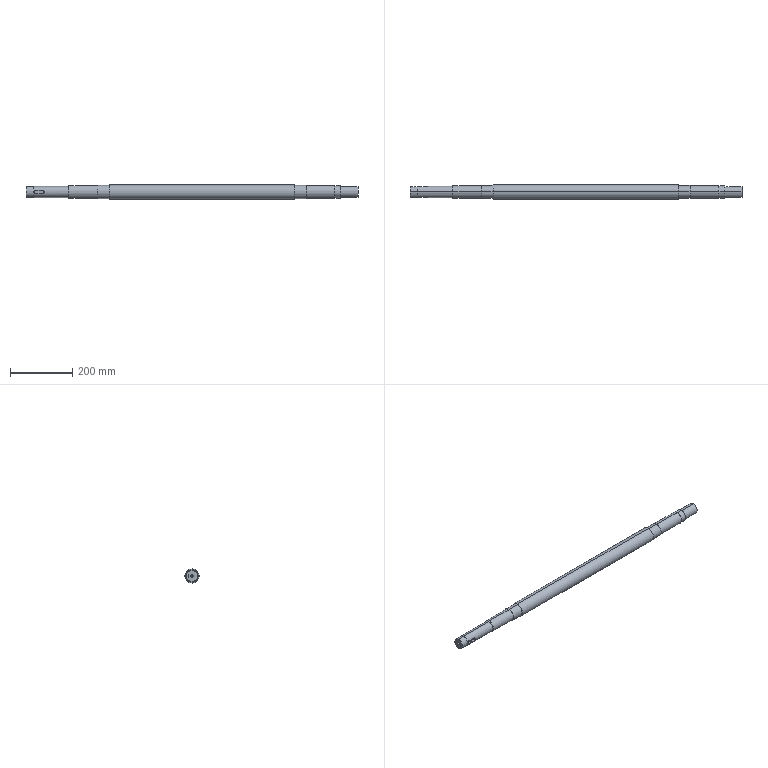Part | SolidWorks | features ICE 11, HoleWzd 2, Extrusion 1, MirrorPattern 1 | 1 solid | 66 faces | box 1067 x 46 x 46 mm | volume 1527789 mm3 | cylinder 34 | plane 28 | cone 4 | commonest cylinder face diameters 10 x8 8.5 x4 12 x4 35 x4 40 x4 42 x4